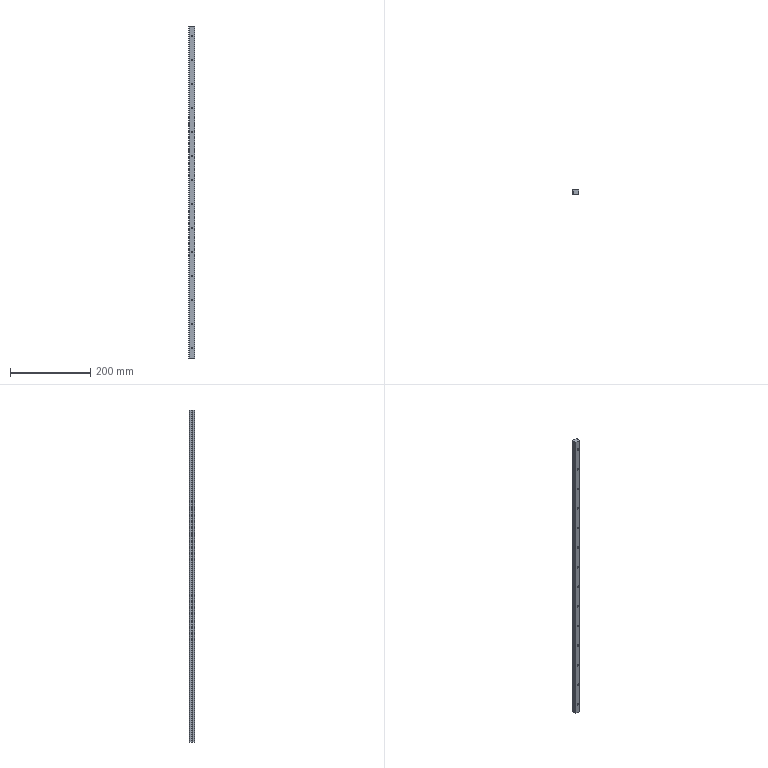Part | STEP file | 1 Rail SSR15XW2SSC1+830LY | 1 solid | 85 faces | box 15 x 12.5 x 830 mm | volume 144164 mm3 | cylinder 63 | plane 22 | commonest cylinder face diameters 4.5 x28 7.5 x28 2 x4 3 x3